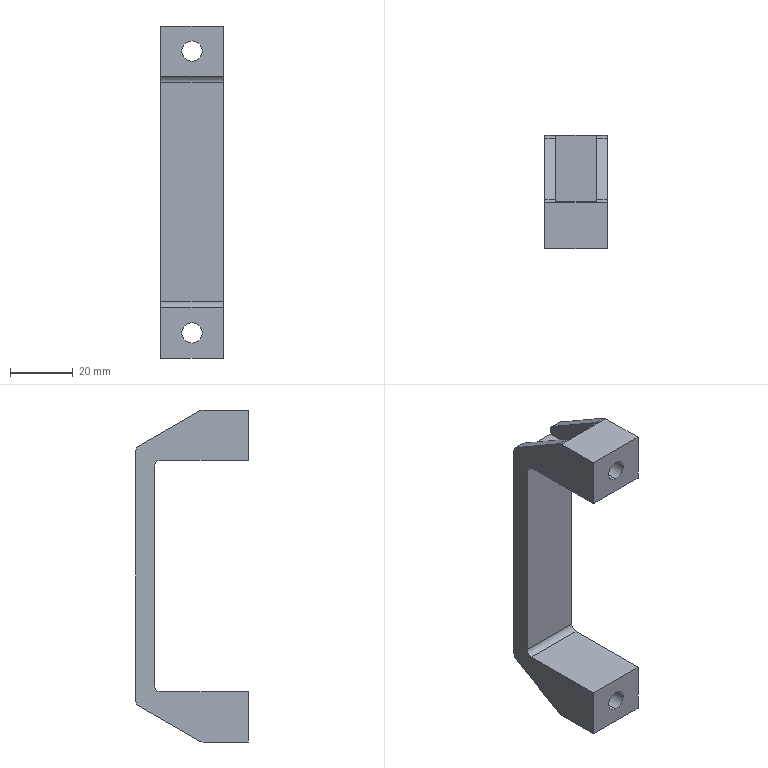Part | SolidWorks | features BaseBody 1 | 1 solid | 40 faces | box 20 x 36 x 106 mm | volume 20303 mm3 | plane 24 | cylinder 16 | commonest cylinder face diameters 4 x8 6.5 x4 11 x4
STEP:
#1=CARTESIAN_POINT('',(10.,15.,50.5));
#2=VERTEX_POINT('',#1);
#3=CARTESIAN_POINT('',(10.,15.,39.5));
#4=VERTEX_POINT('',#3);
#5=CARTESIAN_POINT('',(10.,15.,45.));
#6=DIRECTION('',(0.,-1.,0.));
#7=DIRECTION('',(0.,0.,-1.));
#8=AXIS2_PLACEMENT_3D('',#5,#6,#7);
#9=CIRCLE('',#8,5.5);
#10=EDGE_CURVE('',#2,#4,#9,.T.);
#11=ORIENTED_EDGE('',*,*,#10,.F.);
#12=CARTESIAN_POINT('',(10.,9.5,50.5));
#13=VERTEX_POINT('',#12);
#14=CARTESIAN_POINT('',(10.,15.,50.5));
#15=DIRECTION('',(0.,-1.,0.));
#16=VECTOR('',#15,1000.);
#17=LINE('',#14,#16);
#18=EDGE_CURVE('',#2,#13,#17,.T.);
#19=ORIENTED_EDGE('',*,*,#18,.T.);
#20=CARTESIAN_POINT('',(10.,9.5,39.5));
#21=VERTEX_POINT('',#20);
#22=CARTESIAN_POINT('',(10.,9.5,45.));
#23=DIRECTION('',(0.,1.,0.));
#24=DIRECTION('',(0.,0.,-1.));
#25=AXIS2_PLACEMENT_3D('',#22,#23,#24);
#26=CIRCLE('',#25,5.5);
#27=EDGE_CURVE('',#21,#13,#26,.T.);
#28=ORIENTED_EDGE('',*,*,#27,.F.);
#29=CARTESIAN_POINT('',(10.,15.,39.5));
#30=DIRECTION('',(0.,-1.,0.));
#31=VECTOR('',#30,1000.);
#32=LINE('',#29,#31);
#33=EDGE_CURVE('',#4,#21,#32,.T.);
#34=ORIENTED_EDGE('',*,*,#33,.F.);
#35=EDGE_LOOP('',(#11,#19,#28,#34));
#36=FACE_OUTER_BOUND('',#35,.T.);
#37=CARTESIAN_POINT('',(10.,15.,45.));
#38=DIRECTION('',(0.,-1.,0.));
#39=DIRECTION('',(0.,0.,-1.));
#40=AXIS2_PLACEMENT_3D('',#37,#38,#39);
#41=CYLINDRICAL_SURFACE('',#40,5.5);
#42=ADVANCED_FACE('',(#36),#41,.F.);
#43=CARTESIAN_POINT('',(10.,0.,-41.75));
#44=VERTEX_POINT('',#43);
#45=CARTESIAN_POINT('',(10.,0.,-48.25));
#46=VERTEX_POINT('',#45);
#47=CARTESIAN_POINT('',(10.,0.,-45.));
#48=DIRECTION('',(0.,-1.,0.));
#49=DIRECTION('',(0.,0.,1.));
#50=AXIS2_PLACEMENT_3D('',#47,#48,#49);
#51=CIRCLE('',#50,3.25);
#52=EDGE_CURVE('',#44,#46,#51,.T.);
#53=ORIENTED_EDGE('',*,*,#52,.T.);
#54=CARTESIAN_POINT('',(10.,9.5,-48.25));
#55=VERTEX_POINT('',#54);
#56=CARTESIAN_POINT('',(10.,0.,-48.25));
#57=DIRECTION('',(0.,1.,0.));
#58=VECTOR('',#57,1000.);
#59=LINE('',#56,#58);
#60=EDGE_CURVE('',#46,#55,#59,.T.);
#61=ORIENTED_EDGE('',*,*,#60,.T.);
#62=CARTESIAN_POINT('',(10.,9.5,-41.75));
#63=VERTEX_POINT('',#62);
#64=CARTESIAN_POINT('',(10.,9.5,-45.));
#65=DIRECTION('',(0.,-1.,0.));
#66=DIRECTION('',(0.,0.,1.));
#67=AXIS2_PLACEMENT_3D('',#64,#65,#66);
#68=CIRCLE('',#67,3.25);
#69=EDGE_CURVE('',#63,#55,#68,.T.);
#70=ORIENTED_EDGE('',*,*,#69,.F.);
#71=CARTESIAN_POINT('',(10.,0.,-41.75));
#72=DIRECTION('',(0.,1.,0.));
#73=VECTOR('',#72,1000.);
#74=LINE('',#71,#73);
#75=EDGE_CURVE('',#44,#63,#74,.T.);
#76=ORIENTED_EDGE('',*,*,#75,.F.);
#77=EDGE_LOOP('',(#53,#61,#70,#76));
#78=FACE_OUTER_BOUND('',#77,.T.);
#79=CARTESIAN_POINT('',(10.,0.,-45.));
#80=DIRECTION('',(0.,1.,0.));
#81=DIRECTION('',(0.,0.,1.));
#82=AXIS2_PLACEMENT_3D('',#79,#80,#81);
#83=CYLINDRICAL_SURFACE('',#82,3.25);
#84=ADVANCED_FACE('',(#78),#83,.F.);
#85=CARTESIAN_POINT('',(10.,9.5,48.25));
#86=VERTEX_POINT('',#85);
#87=CARTESIAN_POINT('',(10.,9.5,41.75));
#88=VERTEX_POINT('',#87);
#89=CARTESIAN_POINT('',(10.,9.5,45.));
#90=DIRECTION('',(0.,-1.,0.));
#91=DIRECTION('',(0.,0.,-1.));
#92=AXIS2_PLACEMENT_3D('',#89,#90,#91);
#93=CIRCLE('',#92,3.25);
#94=EDGE_CURVE('',#86,#88,#93,.T.);
#95=ORIENTED_EDGE('',*,*,#94,.F.);
#96=CARTESIAN_POINT('',(10.,0.,48.25));
#97=VERTEX_POINT('',#96);
#98=CARTESIAN_POINT('',(10.,15.,48.25));
#99=DIRECTION('',(0.,-1.,0.));
#100=VECTOR('',#99,1000.);
#101=LINE('',#98,#100);
#102=EDGE_CURVE('',#86,#97,#101,.T.);
#103=ORIENTED_EDGE('',*,*,#102,.T.);
#104=CARTESIAN_POINT('',(10.,0.,41.75));
#105=VERTEX_POINT('',#104);
#106=CARTESIAN_POINT('',(10.,0.,45.));
#107=DIRECTION('',(0.,-1.,0.));
#108=DIRECTION('',(0.,0.,-1.));
#109=AXIS2_PLACEMENT_3D('',#106,#107,#108);
#110=CIRCLE('',#109,3.25);
#111=EDGE_CURVE('',#97,#105,#110,.T.);
#112=ORIENTED_EDGE('',*,*,#111,.T.);
#113=CARTESIAN_POINT('',(10.,15.,41.75));
#114=DIRECTION('',(0.,-1.,0.));
#115=VECTOR('',#114,1000.);
#116=LINE('',#113,#115);
#117=EDGE_CURVE('',#88,#105,#116,.T.);
#118=ORIENTED_EDGE('',*,*,#117,.F.);
#119=EDGE_LOOP('',(#95,#103,#112,#118));
#120=FACE_OUTER_BOUND('',#119,.T.);
#121=CARTESIAN_POINT('',(10.,15.,45.));
#122=DIRECTION('',(0.,-1.,0.));
#123=DIRECTION('',(0.,0.,-1.));
#124=AXIS2_PLACEMENT_3D('',#121,#122,#123);
#125=CYLINDRICAL_SURFACE('',#124,3.25);
#126=ADVANCED_FACE('',(#120),#125,.F.);
#127=CARTESIAN_POINT('',(10.,9.5,-50.5));
#128=VERTEX_POINT('',#127);
#129=CARTESIAN_POINT('',(10.,9.5,-39.5));
#130=VERTEX_POINT('',#129);
#131=CARTESIAN_POINT('',(10.,9.5,-45.));
#132=DIRECTION('',(0.,1.,0.));
#133=DIRECTION('',(0.,0.,1.));
#134=AXIS2_PLACEMENT_3D('',#131,#132,#133);
#135=CIRCLE('',#134,5.5);
#136=EDGE_CURVE('',#128,#130,#135,.T.);
#137=ORIENTED_EDGE('',*,*,#136,.F.);
#138=CARTESIAN_POINT('',(10.,15.,-50.5));
#139=VERTEX_POINT('',#138);
#140=CARTESIAN_POINT('',(10.,0.,-50.5));
#141=DIRECTION('',(0.,1.,0.));
#142=VECTOR('',#141,1000.);
#143=LINE('',#140,#142);
#144=EDGE_CURVE('',#128,#139,#143,.T.);
#145=ORIENTED_EDGE('',*,*,#144,.T.);
#146=CARTESIAN_POINT('',(10.,15.,-39.5));
#147=VERTEX_POINT('',#146);
#148=CARTESIAN_POINT('',(10.,15.,-45.));
#149=DIRECTION('',(0.,-1.,0.));
#150=DIRECTION('',(0.,0.,1.));
#151=AXIS2_PLACEMENT_3D('',#148,#149,#150);
#152=CIRCLE('',#151,5.5);
#153=EDGE_CURVE('',#147,#139,#152,.T.);
#154=ORIENTED_EDGE('',*,*,#153,.F.);
#155=CARTESIAN_POINT('',(10.,0.,-39.5));
#156=DIRECTION('',(0.,1.,0.));
#157=VECTOR('',#156,1000.);
#158=LINE('',#155,#157);
#159=EDGE_CURVE('',#130,#147,#158,.T.);
#160=ORIENTED_EDGE('',*,*,#159,.F.);
#161=EDGE_LOOP('',(#137,#145,#154,#160));
#162=FACE_OUTER_BOUND('',#161,.T.);
#163=CARTESIAN_POINT('',(10.,0.,-45.));
#164=DIRECTION('',(0.,1.,0.));
#165=DIRECTION('',(0.,0.,1.));
#166=AXIS2_PLACEMENT_3D('',#163,#164,#165);
#167=CYLINDRICAL_SURFACE('',#166,5.5);
#168=ADVANCED_FACE('',(#162),#167,.F.);
#169=CARTESIAN_POINT('',(16.5,36.,38.));
#170=VERTEX_POINT('',#169);
#171=CARTESIAN_POINT('',(3.5,36.,38.));
#172=VERTEX_POINT('',#171);
#173=CARTESIAN_POINT('',(20.,36.,38.));
#174=DIRECTION('',(-1.,0.,0.));
#175=VECTOR('',#174,1000.);
#176=LINE('',#173,#175);
#177=EDGE_CURVE('',#170,#172,#176,.T.);
#178=ORIENTED_EDGE('',*,*,#177,.F.);
#179=CARTESIAN_POINT('',(16.5,36.,39.721));
#180=VERTEX_POINT('',#179);
#181=CARTESIAN_POINT('',(16.5,36.,53.));
#182=DIRECTION('',(0.,0.,-1.));
#183=VECTOR('',#182,1000.);
#184=LINE('',#181,#183);
#185=EDGE_CURVE('',#180,#170,#184,.T.);
#186=ORIENTED_EDGE('',*,*,#185,.F.);
#187=CARTESIAN_POINT('',(20.,36.,39.721));
#188=VERTEX_POINT('',#187);
#189=CARTESIAN_POINT('',(20.,36.,39.721));
#190=DIRECTION('',(-1.,0.,0.));
#191=VECTOR('',#190,1000.);
#192=LINE('',#189,#191);
#193=EDGE_CURVE('',#188,#180,#192,.T.);
#194=ORIENTED_EDGE('',*,*,#193,.F.);
#195=CARTESIAN_POINT('',(20.,36.,-39.721));
#196=VERTEX_POINT('',#195);
#197=CARTESIAN_POINT('',(20.,36.,-39.721));
#198=DIRECTION('',(0.,0.,1.));
#199=VECTOR('',#198,1000.);
#200=LINE('',#197,#199);
#201=EDGE_CURVE('',#196,#188,#200,.T.);
#202=ORIENTED_EDGE('',*,*,#201,.F.);
#203=CARTESIAN_POINT('',(16.5,36.,-39.721));
#204=VERTEX_POINT('',#203);
#205=CARTESIAN_POINT('',(20.,36.,-39.721));
#206=DIRECTION('',(1.,0.,0.));
#207=VECTOR('',#206,1000.);
#208=LINE('',#205,#207);
#209=EDGE_CURVE('',#204,#196,#208,.T.);
#210=ORIENTED_EDGE('',*,*,#209,.F.);
#211=CARTESIAN_POINT('',(16.5,36.,-38.));
#212=VERTEX_POINT('',#211);
#213=CARTESIAN_POINT('',(16.5,36.,-38.));
#214=DIRECTION('',(0.,0.,-1.));
#215=VECTOR('',#214,1000.);
#216=LINE('',#213,#215);
#217=EDGE_CURVE('',#212,#204,#216,.T.);
#218=ORIENTED_EDGE('',*,*,#217,.F.);
#219=CARTESIAN_POINT('',(3.5,36.,-38.));
#220=VERTEX_POINT('',#219);
#221=CARTESIAN_POINT('',(20.,36.,-38.));
#222=DIRECTION('',(1.,0.,0.));
#223=VECTOR('',#222,1000.);
#224=LINE('',#221,#223);
#225=EDGE_CURVE('',#220,#212,#224,.T.);
#226=ORIENTED_EDGE('',*,*,#225,.F.);
#227=CARTESIAN_POINT('',(3.5,36.,-39.721));
#228=VERTEX_POINT('',#227);
#229=CARTESIAN_POINT('',(3.5,36.,-53.));
#230=DIRECTION('',(0.,0.,1.));
#231=VECTOR('',#230,1000.);
#232=LINE('',#229,#231);
#233=EDGE_CURVE('',#228,#220,#232,.T.);
#234=ORIENTED_EDGE('',*,*,#233,.F.);
#235=CARTESIAN_POINT('',(0.,36.,-39.721));
#236=VERTEX_POINT('',#235);
#237=CARTESIAN_POINT('',(20.,36.,-39.721));
#238=DIRECTION('',(1.,0.,0.));
#239=VECTOR('',#238,1000.);
#240=LINE('',#237,#239);
#241=EDGE_CURVE('',#236,#228,#240,.T.);
#242=ORIENTED_EDGE('',*,*,#241,.F.);
#243=CARTESIAN_POINT('',(0.,36.,39.721));
#244=VERTEX_POINT('',#243);
#245=CARTESIAN_POINT('',(0.,36.,-39.721));
#246=DIRECTION('',(0.,0.,-1.));
#247=VECTOR('',#246,1000.);
#248=LINE('',#245,#247);
#249=EDGE_CURVE('',#244,#236,#248,.T.);
#250=ORIENTED_EDGE('',*,*,#249,.F.);
#251=CARTESIAN_POINT('',(3.5,36.,39.721));
#252=VERTEX_POINT('',#251);
#253=CARTESIAN_POINT('',(20.,36.,39.721));
#254=DIRECTION('',(-1.,0.,0.));
#255=VECTOR('',#254,1000.);
#256=LINE('',#253,#255);
#257=EDGE_CURVE('',#252,#244,#256,.T.);
#258=ORIENTED_EDGE('',*,*,#257,.F.);
#259=CARTESIAN_POINT('',(3.5,36.,38.));
#260=DIRECTION('',(0.,0.,1.));
#261=VECTOR('',#260,1000.);
#262=LINE('',#259,#261);
#263=EDGE_CURVE('',#172,#252,#262,.T.);
#264=ORIENTED_EDGE('',*,*,#263,.F.);
#265=EDGE_LOOP('',(#178,#186,#194,#202,#210,#218,#226,#234,#242,#250,#258,#264));
#266=FACE_OUTER_BOUND('',#265,.T.);
#267=CARTESIAN_POINT('',(20.,36.,-39.721));
#268=DIRECTION('',(0.,-1.,0.));
#269=DIRECTION('',(0.,0.,-1.));
#270=AXIS2_PLACEMENT_3D('',#267,#268,#269);
#271=PLANE('',#270);
#272=ADVANCED_FACE('',(#266),#271,.F.);
#273=ORIENTED_EDGE('',*,*,#177,.T.);
#274=CARTESIAN_POINT('',(3.5,15.,38.));
#275=VERTEX_POINT('',#274);
#276=CARTESIAN_POINT('',(3.5,36.,38.));
#277=DIRECTION('',(0.,-1.,0.));
#278=VECTOR('',#277,1000.);
#279=LINE('',#276,#278);
#280=EDGE_CURVE('',#172,#275,#279,.T.);
#281=ORIENTED_EDGE('',*,*,#280,.T.);
#282=CARTESIAN_POINT('',(16.5,15.,38.));
#283=VERTEX_POINT('',#282);
#284=CARTESIAN_POINT('',(16.5,15.,38.));
#285=DIRECTION('',(1.,0.,0.));
#286=VECTOR('',#285,1000.);
#287=LINE('',#284,#286);
#288=EDGE_CURVE('',#275,#283,#287,.T.);
#289=ORIENTED_EDGE('',*,*,#288,.T.);
#290=CARTESIAN_POINT('',(16.5,36.,38.));
#291=DIRECTION('',(0.,1.,0.));
#292=VECTOR('',#291,1000.);
#293=LINE('',#290,#292);
#294=EDGE_CURVE('',#283,#170,#293,.T.);
#295=ORIENTED_EDGE('',*,*,#294,.T.);
#296=EDGE_LOOP('',(#273,#281,#289,#295));
#297=FACE_OUTER_BOUND('',#296,.T.);
#298=CARTESIAN_POINT('',(16.5,36.,38.));
#299=DIRECTION('',(0.,0.,1.));
#300=DIRECTION('',(1.,0.,0.));
#301=AXIS2_PLACEMENT_3D('',#298,#299,#300);
#302=PLANE('',#301);
#303=ADVANCED_FACE('',(#297),#302,.T.);
#304=CARTESIAN_POINT('',(20.,35.,41.453));
#305=VERTEX_POINT('',#304);
#306=CARTESIAN_POINT('',(20.,34.,39.721));
#307=DIRECTION('',(-1.,0.,0.));
#308=DIRECTION('',(0.,0.,-1.));
#309=AXIS2_PLACEMENT_3D('',#306,#307,#308);
#310=CIRCLE('',#309,2.);
#311=EDGE_CURVE('',#305,#188,#310,.T.);
#312=ORIENTED_EDGE('',*,*,#311,.T.);
#313=ORIENTED_EDGE('',*,*,#193,.T.);
#314=CARTESIAN_POINT('',(16.5,35.,41.453));
#315=VERTEX_POINT('',#314);
#316=CARTESIAN_POINT('',(16.5,34.,39.721));
#317=DIRECTION('',(1.,0.,0.));
#318=DIRECTION('',(0.,0.,-1.));
#319=AXIS2_PLACEMENT_3D('',#316,#317,#318);
#320=CIRCLE('',#319,2.);
#321=EDGE_CURVE('',#180,#315,#320,.T.);
#322=ORIENTED_EDGE('',*,*,#321,.T.);
#323=CARTESIAN_POINT('',(20.,35.,41.453));
#324=DIRECTION('',(1.,0.,0.));
#325=VECTOR('',#324,1000.);
#326=LINE('',#323,#325);
#327=EDGE_CURVE('',#315,#305,#326,.T.);
#328=ORIENTED_EDGE('',*,*,#327,.T.);
#329=EDGE_LOOP('',(#312,#313,#322,#328));
#330=FACE_OUTER_BOUND('',#329,.T.);
#331=CARTESIAN_POINT('',(20.,34.,39.721));
#332=DIRECTION('',(1.,0.,0.));
#333=DIRECTION('',(0.,0.,-1.));
#334=AXIS2_PLACEMENT_3D('',#331,#332,#333);
#335=CYLINDRICAL_SURFACE('',#334,2.);
#336=ADVANCED_FACE('',(#330),#335,.T.);
#337=ORIENTED_EDGE('',*,*,#311,.F.);
#338=CARTESIAN_POINT('',(20.,15.464,52.732));
#339=VERTEX_POINT('',#338);
#340=CARTESIAN_POINT('',(20.,35.,41.453));
#341=DIRECTION('',(0.,-0.866,0.5));
#342=VECTOR('',#341,1000.);
#343=LINE('',#340,#342);
#344=EDGE_CURVE('',#305,#339,#343,.T.);
#345=ORIENTED_EDGE('',*,*,#344,.T.);
#346=CARTESIAN_POINT('',(20.,14.464,53.));
#347=VERTEX_POINT('',#346);
#348=CARTESIAN_POINT('',(20.,14.464,51.));
#349=DIRECTION('',(-1.,0.,0.));
#350=DIRECTION('',(0.,0.,-1.));
#351=AXIS2_PLACEMENT_3D('',#348,#349,#350);
#352=CIRCLE('',#351,2.);
#353=EDGE_CURVE('',#347,#339,#352,.T.);
#354=ORIENTED_EDGE('',*,*,#353,.F.);
#355=CARTESIAN_POINT('',(20.,0.,53.));
#356=VERTEX_POINT('',#355);
#357=CARTESIAN_POINT('',(20.,14.464,53.));
#358=DIRECTION('',(0.,-1.,0.));
#359=VECTOR('',#358,1000.);
#360=LINE('',#357,#359);
#361=EDGE_CURVE('',#347,#356,#360,.T.);
#362=ORIENTED_EDGE('',*,*,#361,.T.);
#363=CARTESIAN_POINT('',(20.,0.,37.));
#364=VERTEX_POINT('',#363);
#365=CARTESIAN_POINT('',(20.,0.,51.));
#366=DIRECTION('',(0.,0.,-1.));
#367=VECTOR('',#366,1000.);
#368=LINE('',#365,#367);
#369=EDGE_CURVE('',#356,#364,#368,.T.);
#370=ORIENTED_EDGE('',*,*,#369,.T.);
#371=CARTESIAN_POINT('',(20.,28.,37.));
#372=VERTEX_POINT('',#371);
#373=CARTESIAN_POINT('',(20.,14.464,37.));
#374=DIRECTION('',(0.,1.,0.));
#375=VECTOR('',#374,1000.);
#376=LINE('',#373,#375);
#377=EDGE_CURVE('',#364,#372,#376,.T.);
#378=ORIENTED_EDGE('',*,*,#377,.T.);
#379=CARTESIAN_POINT('',(20.,30.,35.));
#380=VERTEX_POINT('',#379);
#381=CARTESIAN_POINT('',(20.,28.,35.));
#382=DIRECTION('',(-1.,0.,0.));
#383=DIRECTION('',(0.,0.,-1.));
#384=AXIS2_PLACEMENT_3D('',#381,#382,#383);
#385=CIRCLE('',#384,2.);
#386=EDGE_CURVE('',#372,#380,#385,.T.);
#387=ORIENTED_EDGE('',*,*,#386,.T.);
#388=CARTESIAN_POINT('',(20.,30.,-35.));
#389=VERTEX_POINT('',#388);
#390=CARTESIAN_POINT('',(20.,30.,51.));
#391=DIRECTION('',(0.,0.,-1.));
#392=VECTOR('',#391,1000.);
#393=LINE('',#390,#392);
#394=EDGE_CURVE('',#380,#389,#393,.T.);
#395=ORIENTED_EDGE('',*,*,#394,.T.);
#396=CARTESIAN_POINT('',(20.,28.,-37.));
#397=VERTEX_POINT('',#396);
#398=CARTESIAN_POINT('',(20.,28.,-35.));
#399=DIRECTION('',(-1.,0.,0.));
#400=DIRECTION('',(0.,0.,-1.));
#401=AXIS2_PLACEMENT_3D('',#398,#399,#400);
#402=CIRCLE('',#401,2.);
#403=EDGE_CURVE('',#389,#397,#402,.T.);
#404=ORIENTED_EDGE('',*,*,#403,.T.);
#405=CARTESIAN_POINT('',(20.,0.,-37.));
#406=VERTEX_POINT('',#405);
#407=CARTESIAN_POINT('',(20.,14.464,-37.));
#408=DIRECTION('',(0.,-1.,0.));
#409=VECTOR('',#408,1000.);
#410=LINE('',#407,#409);
#411=EDGE_CURVE('',#397,#406,#410,.T.);
#412=ORIENTED_EDGE('',*,*,#411,.T.);
#413=CARTESIAN_POINT('',(20.,0.,-53.));
#414=VERTEX_POINT('',#413);
#415=CARTESIAN_POINT('',(20.,0.,51.));
#416=DIRECTION('',(0.,0.,-1.));
#417=VECTOR('',#416,1000.);
#418=LINE('',#415,#417);
#419=EDGE_CURVE('',#406,#414,#418,.T.);
#420=ORIENTED_EDGE('',*,*,#419,.T.);
#421=CARTESIAN_POINT('',(20.,14.464,-53.));
#422=VERTEX_POINT('',#421);
#423=CARTESIAN_POINT('',(20.,14.464,-53.));
#424=DIRECTION('',(0.,1.,0.));
#425=VECTOR('',#424,1000.);
#426=LINE('',#423,#425);
#427=EDGE_CURVE('',#414,#422,#426,.T.);
#428=ORIENTED_EDGE('',*,*,#427,.T.);
#429=CARTESIAN_POINT('',(20.,15.464,-52.732));
#430=VERTEX_POINT('',#429);
#431=CARTESIAN_POINT('',(20.,14.464,-51.));
#432=DIRECTION('',(-1.,0.,0.));
#433=DIRECTION('',(0.,0.,-1.));
#434=AXIS2_PLACEMENT_3D('',#431,#432,#433);
#435=CIRCLE('',#434,2.);
#436=EDGE_CURVE('',#430,#422,#435,.T.);
#437=ORIENTED_EDGE('',*,*,#436,.F.);
#438=CARTESIAN_POINT('',(20.,35.,-41.453));
#439=VERTEX_POINT('',#438);
#440=CARTESIAN_POINT('',(20.,15.464,-52.732));
#441=DIRECTION('',(0.,0.866,0.5));
#442=VECTOR('',#441,1000.);
#443=LINE('',#440,#442);
#444=EDGE_CURVE('',#430,#439,#443,.T.);
#445=ORIENTED_EDGE('',*,*,#444,.T.);
#446=CARTESIAN_POINT('',(20.,34.,-39.721));
#447=DIRECTION('',(1.,0.,0.));
#448=DIRECTION('',(0.,0.,-1.));
#449=AXIS2_PLACEMENT_3D('',#446,#447,#448);
#450=CIRCLE('',#449,2.);
#451=EDGE_CURVE('',#439,#196,#450,.T.);
#452=ORIENTED_EDGE('',*,*,#451,.T.);
#453=ORIENTED_EDGE('',*,*,#201,.T.);
#454=EDGE_LOOP('',(#337,#345,#354,#362,#370,#378,#387,#395,#404,#412,#420,#428,#437,#445,#452,#453));
#455=FACE_OUTER_BOUND('',#454,.T.);
#456=CARTESIAN_POINT('',(20.,14.464,51.));
#457=DIRECTION('',(1.,0.,0.));
#458=DIRECTION('',(0.,0.,-1.));
#459=AXIS2_PLACEMENT_3D('',#456,#457,#458);
#460=PLANE('',#459);
#461=ADVANCED_FACE('',(#455),#460,.T.);
#462=ORIENTED_EDGE('',*,*,#451,.F.);
#463=CARTESIAN_POINT('',(16.5,35.,-41.453));
#464=VERTEX_POINT('',#463);
#465=CARTESIAN_POINT('',(20.,35.,-41.453));
#466=DIRECTION('',(-1.,0.,0.));
#467=VECTOR('',#466,1000.);
#468=LINE('',#465,#467);
#469=EDGE_CURVE('',#439,#464,#468,.T.);
#470=ORIENTED_EDGE('',*,*,#469,.T.);
#471=CARTESIAN_POINT('',(16.5,34.,-39.721));
#472=DIRECTION('',(1.,0.,0.));
#473=DIRECTION('',(0.,0.,-1.));
#474=AXIS2_PLACEMENT_3D('',#471,#472,#473);
#475=CIRCLE('',#474,2.);
#476=EDGE_CURVE('',#464,#204,#475,.T.);
#477=ORIENTED_EDGE('',*,*,#476,.T.);
#478=ORIENTED_EDGE('',*,*,#209,.T.);
#479=EDGE_LOOP('',(#462,#470,#477,#478));
#480=FACE_OUTER_BOUND('',#479,.T.);
#481=CARTESIAN_POINT('',(20.,34.,-39.721));
#482=DIRECTION('',(1.,0.,0.));
#483=DIRECTION('',(0.,0.,-1.));
#484=AXIS2_PLACEMENT_3D('',#481,#482,#483);
#485=CYLINDRICAL_SURFACE('',#484,2.);
#486=ADVANCED_FACE('',(#480),#485,.T.);
#487=ORIENTED_EDGE('',*,*,#225,.T.);
#488=CARTESIAN_POINT('',(16.5,15.,-38.));
#489=VERTEX_POINT('',#488);
#490=CARTESIAN_POINT('',(16.5,36.,-38.));
#491=DIRECTION('',(0.,-1.,0.));
#492=VECTOR('',#491,1000.);
#493=LINE('',#490,#492);
#494=EDGE_CURVE('',#212,#489,#493,.T.);
#495=ORIENTED_EDGE('',*,*,#494,.T.);
#496=CARTESIAN_POINT('',(3.5,15.,-38.));
#497=VERTEX_POINT('',#496);
#498=CARTESIAN_POINT('',(3.5,15.,-38.));
#499=DIRECTION('',(-1.,0.,0.));
#500=VECTOR('',#499,1000.);
#501=LINE('',#498,#500);
#502=EDGE_CURVE('',#489,#497,#501,.T.);
#503=ORIENTED_EDGE('',*,*,#502,.T.);
#504=CARTESIAN_POINT('',(3.5,36.,-38.));
#505=DIRECTION('',(0.,1.,0.));
#506=VECTOR('',#505,1000.);
#507=LINE('',#504,#506);
#508=EDGE_CURVE('',#497,#220,#507,.T.);
#509=ORIENTED_EDGE('',*,*,#508,.T.);
#510=EDGE_LOOP('',(#487,#495,#503,#509));
#511=FACE_OUTER_BOUND('',#510,.T.);
#512=CARTESIAN_POINT('',(3.5,36.,-38.));
#513=DIRECTION('',(0.,0.,-1.));
#514=DIRECTION('',(-1.,0.,0.));
#515=AXIS2_PLACEMENT_3D('',#512,#513,#514);
#516=PLANE('',#515);
#517=ADVANCED_FACE('',(#511),#516,.T.);
#518=CARTESIAN_POINT('',(0.,35.,-41.453));
#519=VERTEX_POINT('',#518);
#520=CARTESIAN_POINT('',(0.,34.,-39.721));
#521=DIRECTION('',(1.,0.,0.));
#522=DIRECTION('',(0.,0.,-1.));
#523=AXIS2_PLACEMENT_3D('',#520,#521,#522);
#524=CIRCLE('',#523,2.);
#525=EDGE_CURVE('',#519,#236,#524,.T.);
#526=ORIENTED_EDGE('',*,*,#525,.T.);
#527=ORIENTED_EDGE('',*,*,#241,.T.);
#528=CARTESIAN_POINT('',(3.5,35.,-41.453));
#529=VERTEX_POINT('',#528);
#530=CARTESIAN_POINT('',(3.5,34.,-39.721));
#531=DIRECTION('',(-1.,0.,0.));
#532=DIRECTION('',(0.,0.,-1.));
#533=AXIS2_PLACEMENT_3D('',#530,#531,#532);
#534=CIRCLE('',#533,2.);
#535=EDGE_CURVE('',#228,#529,#534,.T.);
#536=ORIENTED_EDGE('',*,*,#535,.T.);
#537=CARTESIAN_POINT('',(20.,35.,-41.453));
#538=DIRECTION('',(-1.,0.,0.));
#539=VECTOR('',#538,1000.);
#540=LINE('',#537,#539);
#541=EDGE_CURVE('',#529,#519,#540,.T.);
#542=ORIENTED_EDGE('',*,*,#541,.T.);
#543=EDGE_LOOP('',(#526,#527,#536,#542));
#544=FACE_OUTER_BOUND('',#543,.T.);
#545=CARTESIAN_POINT('',(20.,34.,-39.721));
#546=DIRECTION('',(1.,0.,0.));
#547=DIRECTION('',(0.,0.,-1.));
#548=AXIS2_PLACEMENT_3D('',#545,#546,#547);
#549=CYLINDRICAL_SURFACE('',#548,2.);
#550=ADVANCED_FACE('',(#544),#549,.T.);
#551=CARTESIAN_POINT('',(0.,35.,41.453));
#552=VERTEX_POINT('',#551);
#553=CARTESIAN_POINT('',(0.,15.464,52.732));
#554=VERTEX_POINT('',#553);
#555=CARTESIAN_POINT('',(0.,35.,41.453));
#556=DIRECTION('',(0.,-0.866,0.5));
#557=VECTOR('',#556,1000.);
#558=LINE('',#555,#557);
#559=EDGE_CURVE('',#552,#554,#558,.T.);
#560=ORIENTED_EDGE('',*,*,#559,.F.);
#561=CARTESIAN_POINT('',(0.,34.,39.721));
#562=DIRECTION('',(1.,0.,0.));
#563=DIRECTION('',(0.,0.,-1.));
#564=AXIS2_PLACEMENT_3D('',#561,#562,#563);
#565=CIRCLE('',#564,2.);
#566=EDGE_CURVE('',#244,#552,#565,.T.);
#567=ORIENTED_EDGE('',*,*,#566,.F.);
#568=ORIENTED_EDGE('',*,*,#249,.T.);
#569=ORIENTED_EDGE('',*,*,#525,.F.);
#570=CARTESIAN_POINT('',(0.,15.464,-52.732));
#571=VERTEX_POINT('',#570);
#572=CARTESIAN_POINT('',(0.,15.464,-52.732));
#573=DIRECTION('',(0.,0.866,0.5));
#574=VECTOR('',#573,1000.);
#575=LINE('',#572,#574);
#576=EDGE_CURVE('',#571,#519,#575,.T.);
#577=ORIENTED_EDGE('',*,*,#576,.F.);
#578=CARTESIAN_POINT('',(0.,14.464,-53.));
#579=VERTEX_POINT('',#578);
#580=CARTESIAN_POINT('',(0.,14.464,-51.));
#581=DIRECTION('',(1.,0.,0.));
#582=DIRECTION('',(0.,0.,-1.));
#583=AXIS2_PLACEMENT_3D('',#580,#581,#582);
#584=CIRCLE('',#583,2.);
#585=EDGE_CURVE('',#579,#571,#584,.T.);
#586=ORIENTED_EDGE('',*,*,#585,.F.);
#587=CARTESIAN_POINT('',(0.,0.,-53.));
#588=VERTEX_POINT('',#587);
#589=CARTESIAN_POINT('',(0.,14.464,-53.));
#590=DIRECTION('',(0.,1.,0.));
#591=VECTOR('',#590,1000.);
#592=LINE('',#589,#591);
#593=EDGE_CURVE('',#588,#579,#592,.T.);
#594=ORIENTED_EDGE('',*,*,#593,.F.);
#595=CARTESIAN_POINT('',(0.,0.,-37.));
#596=VERTEX_POINT('',#595);
#597=CARTESIAN_POINT('',(0.,0.,51.));
#598=DIRECTION('',(0.,0.,-1.));
#599=VECTOR('',#598,1000.);
#600=LINE('',#597,#599);
#601=EDGE_CURVE('',#596,#588,#600,.T.);
#602=ORIENTED_EDGE('',*,*,#601,.F.);
#603=CARTESIAN_POINT('',(0.,28.,-37.));
#604=VERTEX_POINT('',#603);
#605=CARTESIAN_POINT('',(0.,14.464,-37.));
#606=DIRECTION('',(0.,-1.,0.));
#607=VECTOR('',#606,1000.);
#608=LINE('',#605,#607);
#609=EDGE_CURVE('',#604,#596,#608,.T.);
#610=ORIENTED_EDGE('',*,*,#609,.F.);
#611=CARTESIAN_POINT('',(0.,30.,-35.));
#612=VERTEX_POINT('',#611);
#613=CARTESIAN_POINT('',(0.,28.,-35.));
#614=DIRECTION('',(-1.,0.,0.));
#615=DIRECTION('',(0.,0.,-1.));
#616=AXIS2_PLACEMENT_3D('',#613,#614,#615);
#617=CIRCLE('',#616,2.);
#618=EDGE_CURVE('',#612,#604,#617,.T.);
#619=ORIENTED_EDGE('',*,*,#618,.F.);
#620=CARTESIAN_POINT('',(0.,30.,35.));
#621=VERTEX_POINT('',#620);
#622=CARTESIAN_POINT('',(0.,30.,51.));
#623=DIRECTION('',(0.,0.,-1.));
#624=VECTOR('',#623,1000.);
#625=LINE('',#622,#624);
#626=EDGE_CURVE('',#621,#612,#625,.T.);
#627=ORIENTED_EDGE('',*,*,#626,.F.);
#628=CARTESIAN_POINT('',(0.,28.,37.));
#629=VERTEX_POINT('',#628);
#630=CARTESIAN_POINT('',(0.,28.,35.));
#631=DIRECTION('',(-1.,0.,0.));
#632=DIRECTION('',(0.,0.,-1.));
#633=AXIS2_PLACEMENT_3D('',#630,#631,#632);
#634=CIRCLE('',#633,2.);
#635=EDGE_CURVE('',#629,#621,#634,.T.);
#636=ORIENTED_EDGE('',*,*,#635,.F.);
#637=CARTESIAN_POINT('',(0.,0.,37.));
#638=VERTEX_POINT('',#637);
#639=CARTESIAN_POINT('',(0.,14.464,37.));
#640=DIRECTION('',(0.,1.,0.));
#641=VECTOR('',#640,1000.);
#642=LINE('',#639,#641);
#643=EDGE_CURVE('',#638,#629,#642,.T.);
#644=ORIENTED_EDGE('',*,*,#643,.F.);
#645=CARTESIAN_POINT('',(0.,0.,53.));
#646=VERTEX_POINT('',#645);
#647=CARTESIAN_POINT('',(0.,0.,51.));
#648=DIRECTION('',(0.,0.,-1.));
#649=VECTOR('',#648,1000.);
#650=LINE('',#647,#649);
#651=EDGE_CURVE('',#646,#638,#650,.T.);
#652=ORIENTED_EDGE('',*,*,#651,.F.);
#653=CARTESIAN_POINT('',(0.,14.464,53.));
#654=VERTEX_POINT('',#653);
#655=CARTESIAN_POINT('',(0.,14.464,53.));
#656=DIRECTION('',(0.,-1.,0.));
#657=VECTOR('',#656,1000.);
#658=LINE('',#655,#657);
#659=EDGE_CURVE('',#654,#646,#658,.T.);
#660=ORIENTED_EDGE('',*,*,#659,.F.);
#661=CARTESIAN_POINT('',(0.,14.464,51.));
#662=DIRECTION('',(1.,0.,0.));
#663=DIRECTION('',(0.,0.,-1.));
#664=AXIS2_PLACEMENT_3D('',#661,#662,#663);
#665=CIRCLE('',#664,2.);
#666=EDGE_CURVE('',#554,#654,#665,.T.);
#667=ORIENTED_EDGE('',*,*,#666,.F.);
#668=EDGE_LOOP('',(#560,#567,#568,#569,#577,#586,#594,#602,#610,#619,#627,#636,#644,#652,#660,#667));
#669=FACE_OUTER_BOUND('',#668,.T.);
#670=CARTESIAN_POINT('',(0.,14.464,51.));
#671=DIRECTION('',(1.,0.,0.));
#672=DIRECTION('',(0.,0.,-1.));
#673=AXIS2_PLACEMENT_3D('',#670,#671,#672);
#674=PLANE('',#673);
#675=ADVANCED_FACE('',(#669),#674,.F.);
#676=ORIENTED_EDGE('',*,*,#566,.T.);
#677=CARTESIAN_POINT('',(3.5,35.,41.453));
#678=VERTEX_POINT('',#677);
#679=CARTESIAN_POINT('',(20.,35.,41.453));
#680=DIRECTION('',(1.,0.,0.));
#681=VECTOR('',#680,1000.);
#682=LINE('',#679,#681);
#683=EDGE_CURVE('',#552,#678,#682,.T.);
#684=ORIENTED_EDGE('',*,*,#683,.T.);
#685=CARTESIAN_POINT('',(3.5,34.,39.721));
#686=DIRECTION('',(-1.,0.,0.));
#687=DIRECTION('',(0.,0.,-1.));
#688=AXIS2_PLACEMENT_3D('',#685,#686,#687);
#689=CIRCLE('',#688,2.);
#690=EDGE_CURVE('',#678,#252,#689,.T.);
#691=ORIENTED_EDGE('',*,*,#690,.T.);
#692=ORIENTED_EDGE('',*,*,#257,.T.);
#693=EDGE_LOOP('',(#676,#684,#691,#692));
#694=FACE_OUTER_BOUND('',#693,.T.);
#695=CARTESIAN_POINT('',(20.,34.,39.721));
#696=DIRECTION('',(1.,0.,0.));
#697=DIRECTION('',(0.,0.,-1.));
#698=AXIS2_PLACEMENT_3D('',#695,#696,#697);
#699=CYLINDRICAL_SURFACE('',#698,2.);
#700=ADVANCED_FACE('',(#694),#699,.T.);
#701=ORIENTED_EDGE('',*,*,#690,.F.);
#702=CARTESIAN_POINT('',(3.5,15.464,52.732));
#703=VERTEX_POINT('',#702);
#704=CARTESIAN_POINT('',(3.5,35.,41.453));
#705=DIRECTION('',(0.,-0.866,0.5));
#706=VECTOR('',#705,1000.);
#707=LINE('',#704,#706);
#708=EDGE_CURVE('',#678,#703,#707,.T.);
#709=ORIENTED_EDGE('',*,*,#708,.T.);
#710=CARTESIAN_POINT('',(3.5,15.,52.927));
#711=VERTEX_POINT('',#710);
#712=CARTESIAN_POINT('',(3.5,14.464,51.));
#713=DIRECTION('',(-1.,0.,0.));
#714=DIRECTION('',(0.,0.,-1.));
#715=AXIS2_PLACEMENT_3D('',#712,#713,#714);
#716=CIRCLE('',#715,2.);
#717=EDGE_CURVE('',#711,#703,#716,.T.);
#718=ORIENTED_EDGE('',*,*,#717,.F.);
#719=CARTESIAN_POINT('',(3.5,15.,38.));
#720=DIRECTION('',(0.,0.,-1.));
#721=VECTOR('',#720,1000.);
#722=LINE('',#719,#721);
#723=EDGE_CURVE('',#711,#275,#722,.T.);
#724=ORIENTED_EDGE('',*,*,#723,.T.);
#725=ORIENTED_EDGE('',*,*,#280,.F.);
#726=ORIENTED_EDGE('',*,*,#263,.T.);
#727=EDGE_LOOP('',(#701,#709,#718,#724,#725,#726));
#728=FACE_OUTER_BOUND('',#727,.T.);
#729=CARTESIAN_POINT('',(3.5,36.,38.));
#730=DIRECTION('',(1.,0.,0.));
#731=DIRECTION('',(0.,0.,-1.));
#732=AXIS2_PLACEMENT_3D('',#729,#730,#731);
#733=PLANE('',#732);
#734=ADVANCED_FACE('',(#728),#733,.T.);
#735=ORIENTED_EDGE('',*,*,#294,.F.);
#736=CARTESIAN_POINT('',(16.5,15.,52.927));
#737=VERTEX_POINT('',#736);
#738=CARTESIAN_POINT('',(16.5,15.,53.));
#739=DIRECTION('',(0.,0.,1.));
#740=VECTOR('',#739,1000.);
#741=LINE('',#738,#740);
#742=EDGE_CURVE('',#283,#737,#741,.T.);
#743=ORIENTED_EDGE('',*,*,#742,.T.);
#744=CARTESIAN_POINT('',(16.5,15.464,52.732));
#745=VERTEX_POINT('',#744);
#746=CARTESIAN_POINT('',(16.5,14.464,51.));
#747=DIRECTION('',(1.,0.,0.));
#748=DIRECTION('',(0.,0.,-1.));
#749=AXIS2_PLACEMENT_3D('',#746,#747,#748);
#750=CIRCLE('',#749,2.);
#751=EDGE_CURVE('',#745,#737,#750,.T.);
#752=ORIENTED_EDGE('',*,*,#751,.F.);
#753=CARTESIAN_POINT('',(16.5,15.464,52.732));
#754=DIRECTION('',(0.,0.866,-0.5));
#755=VECTOR('',#754,1000.);
#756=LINE('',#753,#755);
#757=EDGE_CURVE('',#745,#315,#756,.T.);
#758=ORIENTED_EDGE('',*,*,#757,.T.);
#759=ORIENTED_EDGE('',*,*,#321,.F.);
#760=ORIENTED_EDGE('',*,*,#185,.T.);
#761=EDGE_LOOP('',(#735,#743,#752,#758,#759,#760));
#762=FACE_OUTER_BOUND('',#761,.T.);
#763=CARTESIAN_POINT('',(16.5,36.,53.));
#764=DIRECTION('',(-1.,0.,0.));
#765=DIRECTION('',(0.,0.,1.));
#766=AXIS2_PLACEMENT_3D('',#763,#764,#765);
#767=PLANE('',#766);
#768=ADVANCED_FACE('',(#762),#767,.T.);
#769=ORIENTED_EDGE('',*,*,#288,.F.);
#770=ORIENTED_EDGE('',*,*,#723,.F.);
#771=CARTESIAN_POINT('',(0.,15.,52.927));
#772=DIRECTION('',(1.,0.,0.));
#773=VECTOR('',#772,1000.);
#774=LINE('',#771,#773);
#775=EDGE_CURVE('',#711,#737,#774,.T.);
#776=ORIENTED_EDGE('',*,*,#775,.T.);
#777=ORIENTED_EDGE('',*,*,#742,.F.);
#778=EDGE_LOOP('',(#769,#770,#776,#777));
#779=FACE_OUTER_BOUND('',#778,.T.);
#780=CARTESIAN_POINT('',(10.,15.,45.));
#781=DIRECTION('',(0.,-1.,0.));
#782=DIRECTION('',(0.,0.,-1.));
#783=AXIS2_PLACEMENT_3D('',#780,#781,#782);
#784=CIRCLE('',#783,5.5);
#785=EDGE_CURVE('',#4,#2,#784,.T.);
#786=ORIENTED_EDGE('',*,*,#785,.T.);
#787=ORIENTED_EDGE('',*,*,#10,.T.);
#788=EDGE_LOOP('',(#786,#787));
#789=FACE_BOUND('',#788,.T.);
#790=CARTESIAN_POINT('',(0.,15.,0.));
#791=DIRECTION('',(0.,1.,0.));
#792=DIRECTION('',(0.,0.,1.));
#793=AXIS2_PLACEMENT_3D('',#790,#791,#792);
#794=PLANE('',#793);
#795=ADVANCED_FACE('',(#779,#789),#794,.T.);
#796=CARTESIAN_POINT('',(20.,15.464,52.732));
#797=DIRECTION('',(-1.,0.,0.));
#798=VECTOR('',#797,1000.);
#799=LINE('',#796,#798);
#800=EDGE_CURVE('',#339,#745,#799,.T.);
#801=ORIENTED_EDGE('',*,*,#800,.F.);
#802=ORIENTED_EDGE('',*,*,#344,.F.);
#803=ORIENTED_EDGE('',*,*,#327,.F.);
#804=ORIENTED_EDGE('',*,*,#757,.F.);
#805=EDGE_LOOP('',(#801,#802,#803,#804));
#806=FACE_OUTER_BOUND('',#805,.T.);
#807=CARTESIAN_POINT('',(20.,35.,41.453));
#808=DIRECTION('',(0.,-0.5,-0.866));
#809=DIRECTION('',(0.,0.866,-0.5));
#810=AXIS2_PLACEMENT_3D('',#807,#808,#809);
#811=PLANE('',#810);
#812=ADVANCED_FACE('',(#806),#811,.F.);
#813=ORIENTED_EDGE('',*,*,#469,.F.);
#814=ORIENTED_EDGE('',*,*,#444,.F.);
#815=CARTESIAN_POINT('',(16.5,15.464,-52.732));
#816=VERTEX_POINT('',#815);
#817=CARTESIAN_POINT('',(20.,15.464,-52.732));
#818=DIRECTION('',(1.,0.,0.));
#819=VECTOR('',#818,1000.);
#820=LINE('',#817,#819);
#821=EDGE_CURVE('',#816,#430,#820,.T.);
#822=ORIENTED_EDGE('',*,*,#821,.F.);
#823=CARTESIAN_POINT('',(16.5,15.464,-52.732));
#824=DIRECTION('',(0.,-0.866,-0.5));
#825=VECTOR('',#824,1000.);
#826=LINE('',#823,#825);
#827=EDGE_CURVE('',#464,#816,#826,.T.);
#828=ORIENTED_EDGE('',*,*,#827,.F.);
#829=EDGE_LOOP('',(#813,#814,#822,#828));
#830=FACE_OUTER_BOUND('',#829,.T.);
#831=CARTESIAN_POINT('',(20.,15.464,-52.732));
#832=DIRECTION('',(0.,-0.5,0.866));
#833=DIRECTION('',(0.,-0.866,-0.5));
#834=AXIS2_PLACEMENT_3D('',#831,#832,#833);
#835=PLANE('',#834);
#836=ADVANCED_FACE('',(#830),#835,.F.);
#837=CARTESIAN_POINT('',(20.,14.464,-53.));
#838=DIRECTION('',(-1.,0.,0.));
#839=VECTOR('',#838,1000.);
#840=LINE('',#837,#839);
#841=EDGE_CURVE('',#422,#579,#840,.T.);
#842=ORIENTED_EDGE('',*,*,#841,.F.);
#843=ORIENTED_EDGE('',*,*,#427,.F.);
#844=CARTESIAN_POINT('',(20.,0.,-53.));
#845=DIRECTION('',(1.,0.,0.));
#846=VECTOR('',#845,1000.);
#847=LINE('',#844,#846);
#848=EDGE_CURVE('',#588,#414,#847,.T.);
#849=ORIENTED_EDGE('',*,*,#848,.F.);
#850=ORIENTED_EDGE('',*,*,#593,.T.);
#851=EDGE_LOOP('',(#842,#843,#849,#850));
#852=FACE_OUTER_BOUND('',#851,.T.);
#853=CARTESIAN_POINT('',(20.,0.,-53.));
#854=DIRECTION('',(0.,0.,1.));
#855=DIRECTION('',(1.,0.,0.));
#856=AXIS2_PLACEMENT_3D('',#853,#854,#855);
#857=PLANE('',#856);
#858=ADVANCED_FACE('',(#852),#857,.F.);
#859=ORIENTED_EDGE('',*,*,#848,.T.);
#860=ORIENTED_EDGE('',*,*,#419,.F.);
#861=CARTESIAN_POINT('',(20.,0.,-37.));
#862=DIRECTION('',(1.,0.,0.));
#863=VECTOR('',#862,1000.);
#864=LINE('',#861,#863);
#865=EDGE_CURVE('',#596,#406,#864,.T.);
#866=ORIENTED_EDGE('',*,*,#865,.F.);
#867=ORIENTED_EDGE('',*,*,#601,.T.);
#868=EDGE_LOOP('',(#859,#860,#866,#867));
#869=FACE_OUTER_BOUND('',#868,.T.);
#870=ORIENTED_EDGE('',*,*,#52,.F.);
#871=CARTESIAN_POINT('',(10.,0.,-45.));
#872=DIRECTION('',(0.,-1.,0.));
#873=DIRECTION('',(0.,0.,1.));
#874=AXIS2_PLACEMENT_3D('',#871,#872,#873);
#875=CIRCLE('',#874,3.25);
#876=EDGE_CURVE('',#46,#44,#875,.T.);
#877=ORIENTED_EDGE('',*,*,#876,.F.);
#878=EDGE_LOOP('',(#870,#877));
#879=FACE_BOUND('',#878,.T.);
#880=CARTESIAN_POINT('',(20.,0.,-37.));
#881=DIRECTION('',(0.,1.,0.));
#882=DIRECTION('',(0.,0.,1.));
#883=AXIS2_PLACEMENT_3D('',#880,#881,#882);
#884=PLANE('',#883);
#885=ADVANCED_FACE('',(#869,#879),#884,.F.);
#886=ORIENTED_EDGE('',*,*,#865,.T.);
#887=ORIENTED_EDGE('',*,*,#411,.F.);
#888=CARTESIAN_POINT('',(20.,28.,-37.));
#889=DIRECTION('',(1.,0.,0.));
#890=VECTOR('',#889,1000.);
#891=LINE('',#888,#890);
#892=EDGE_CURVE('',#604,#397,#891,.T.);
#893=ORIENTED_EDGE('',*,*,#892,.F.);
#894=ORIENTED_EDGE('',*,*,#609,.T.);
#895=EDGE_LOOP('',(#886,#887,#893,#894));
#896=FACE_OUTER_BOUND('',#895,.T.);
#897=CARTESIAN_POINT('',(20.,28.,-37.));
#898=DIRECTION('',(0.,0.,-1.));
#899=DIRECTION('',(-1.,0.,0.));
#900=AXIS2_PLACEMENT_3D('',#897,#898,#899);
#901=PLANE('',#900);
#902=ADVANCED_FACE('',(#896),#901,.F.);
#903=ORIENTED_EDGE('',*,*,#892,.T.);
#904=ORIENTED_EDGE('',*,*,#403,.F.);
#905=CARTESIAN_POINT('',(20.,30.,-35.));
#906=DIRECTION('',(1.,0.,0.));
#907=VECTOR('',#906,1000.);
#908=LINE('',#905,#907);
#909=EDGE_CURVE('',#612,#389,#908,.T.);
#910=ORIENTED_EDGE('',*,*,#909,.F.);
#911=ORIENTED_EDGE('',*,*,#618,.T.);
#912=EDGE_LOOP('',(#903,#904,#910,#911));
#913=FACE_OUTER_BOUND('',#912,.T.);
#914=CARTESIAN_POINT('',(20.,28.,-35.));
#915=DIRECTION('',(1.,0.,0.));
#916=DIRECTION('',(0.,0.,-1.));
#917=AXIS2_PLACEMENT_3D('',#914,#915,#916);
#918=CYLINDRICAL_SURFACE('',#917,2.);
#919=ADVANCED_FACE('',(#913),#918,.F.);
#920=ORIENTED_EDGE('',*,*,#909,.T.);
#921=ORIENTED_EDGE('',*,*,#394,.F.);
#922=CARTESIAN_POINT('',(20.,30.,35.));
#923=DIRECTION('',(1.,0.,0.));
#924=VECTOR('',#923,1000.);
#925=LINE('',#922,#924);
#926=EDGE_CURVE('',#621,#380,#925,.T.);
#927=ORIENTED_EDGE('',*,*,#926,.F.);
#928=ORIENTED_EDGE('',*,*,#626,.T.);
#929=EDGE_LOOP('',(#920,#921,#927,#928));
#930=FACE_OUTER_BOUND('',#929,.T.);
#931=CARTESIAN_POINT('',(20.,30.,35.));
#932=DIRECTION('',(0.,1.,0.));
#933=DIRECTION('',(0.,0.,1.));
#934=AXIS2_PLACEMENT_3D('',#931,#932,#933);
#935=PLANE('',#934);
#936=ADVANCED_FACE('',(#930),#935,.F.);
#937=ORIENTED_EDGE('',*,*,#926,.T.);
#938=ORIENTED_EDGE('',*,*,#386,.F.);
#939=CARTESIAN_POINT('',(20.,28.,37.));
#940=DIRECTION('',(1.,0.,0.));
#941=VECTOR('',#940,1000.);
#942=LINE('',#939,#941);
#943=EDGE_CURVE('',#629,#372,#942,.T.);
#944=ORIENTED_EDGE('',*,*,#943,.F.);
#945=ORIENTED_EDGE('',*,*,#635,.T.);
#946=EDGE_LOOP('',(#937,#938,#944,#945));
#947=FACE_OUTER_BOUND('',#946,.T.);
#948=CARTESIAN_POINT('',(20.,28.,35.));
#949=DIRECTION('',(1.,0.,0.));
#950=DIRECTION('',(0.,0.,-1.));
#951=AXIS2_PLACEMENT_3D('',#948,#949,#950);
#952=CYLINDRICAL_SURFACE('',#951,2.);
#953=ADVANCED_FACE('',(#947),#952,.F.);
#954=ORIENTED_EDGE('',*,*,#943,.T.);
#955=ORIENTED_EDGE('',*,*,#377,.F.);
#956=CARTESIAN_POINT('',(20.,0.,37.));
#957=DIRECTION('',(1.,0.,0.));
#958=VECTOR('',#957,1000.);
#959=LINE('',#956,#958);
#960=EDGE_CURVE('',#638,#364,#959,.T.);
#961=ORIENTED_EDGE('',*,*,#960,.F.);
#962=ORIENTED_EDGE('',*,*,#643,.T.);
#963=EDGE_LOOP('',(#954,#955,#961,#962));
#964=FACE_OUTER_BOUND('',#963,.T.);
#965=CARTESIAN_POINT('',(20.,0.,37.));
#966=DIRECTION('',(0.,0.,1.));
#967=DIRECTION('',(1.,0.,0.));
#968=AXIS2_PLACEMENT_3D('',#965,#966,#967);
#969=PLANE('',#968);
#970=ADVANCED_FACE('',(#964),#969,.F.);
#971=ORIENTED_EDGE('',*,*,#960,.T.);
#972=ORIENTED_EDGE('',*,*,#369,.F.);
#973=CARTESIAN_POINT('',(20.,0.,53.));
#974=DIRECTION('',(1.,0.,0.));
#975=VECTOR('',#974,1000.);
#976=LINE('',#973,#975);
#977=EDGE_CURVE('',#646,#356,#976,.T.);
#978=ORIENTED_EDGE('',*,*,#977,.F.);
#979=ORIENTED_EDGE('',*,*,#651,.T.);
#980=EDGE_LOOP('',(#971,#972,#978,#979));
#981=FACE_OUTER_BOUND('',#980,.T.);
#982=CARTESIAN_POINT('',(10.,0.,45.));
#983=DIRECTION('',(0.,-1.,0.));
#984=DIRECTION('',(0.,0.,-1.));
#985=AXIS2_PLACEMENT_3D('',#982,#983,#984);
#986=CIRCLE('',#985,3.25);
#987=EDGE_CURVE('',#105,#97,#986,.T.);
#988=ORIENTED_EDGE('',*,*,#987,.F.);
#989=ORIENTED_EDGE('',*,*,#111,.F.);
#990=EDGE_LOOP('',(#988,#989));
#991=FACE_BOUND('',#990,.T.);
#992=CARTESIAN_POINT('',(20.,0.,53.));
#993=DIRECTION('',(0.,1.,0.));
#994=DIRECTION('',(0.,0.,1.));
#995=AXIS2_PLACEMENT_3D('',#992,#993,#994);
#996=PLANE('',#995);
#997=ADVANCED_FACE('',(#981,#991),#996,.F.);
#998=ORIENTED_EDGE('',*,*,#977,.T.);
#999=ORIENTED_EDGE('',*,*,#361,.F.);
#1000=CARTESIAN_POINT('',(20.,14.464,53.));
#1001=DIRECTION('',(1.,0.,0.));
#1002=VECTOR('',#1001,1000.);
#1003=LINE('',#1000,#1002);
#1004=EDGE_CURVE('',#654,#347,#1003,.T.);
#1005=ORIENTED_EDGE('',*,*,#1004,.F.);
#1006=ORIENTED_EDGE('',*,*,#659,.T.);
#1007=EDGE_LOOP('',(#998,#999,#1005,#1006));
#1008=FACE_OUTER_BOUND('',#1007,.T.);
#1009=CARTESIAN_POINT('',(20.,14.464,53.));
#1010=DIRECTION('',(0.,0.,-1.));
#1011=DIRECTION('',(-1.,0.,0.));
#1012=AXIS2_PLACEMENT_3D('',#1009,#1010,#1011);
#1013=PLANE('',#1012);
#1014=ADVANCED_FACE('',(#1008),#1013,.F.);
#1015=ORIENTED_EDGE('',*,*,#476,.F.);
#1016=ORIENTED_EDGE('',*,*,#827,.T.);
#1017=CARTESIAN_POINT('',(16.5,15.,-52.927));
#1018=VERTEX_POINT('',#1017);
#1019=CARTESIAN_POINT('',(16.5,14.464,-51.));
#1020=DIRECTION('',(-1.,0.,0.));
#1021=DIRECTION('',(0.,0.,-1.));
#1022=AXIS2_PLACEMENT_3D('',#1019,#1020,#1021);
#1023=CIRCLE('',#1022,2.);
#1024=EDGE_CURVE('',#816,#1018,#1023,.T.);
#1025=ORIENTED_EDGE('',*,*,#1024,.T.);
#1026=CARTESIAN_POINT('',(16.5,15.,-38.));
#1027=DIRECTION('',(0.,0.,1.));
#1028=VECTOR('',#1027,1000.);
#1029=LINE('',#1026,#1028);
#1030=EDGE_CURVE('',#1018,#489,#1029,.T.);
#1031=ORIENTED_EDGE('',*,*,#1030,.T.);
#1032=ORIENTED_EDGE('',*,*,#494,.F.);
#1033=ORIENTED_EDGE('',*,*,#217,.T.);
#1034=EDGE_LOOP('',(#1015,#1016,#1025,#1031,#1032,#1033));
#1035=FACE_OUTER_BOUND('',#1034,.T.);
#1036=CARTESIAN_POINT('',(16.5,36.,-38.));
#1037=DIRECTION('',(-1.,0.,0.));
#1038=DIRECTION('',(0.,0.,1.));
#1039=AXIS2_PLACEMENT_3D('',#1036,#1037,#1038);
#1040=PLANE('',#1039);
#1041=ADVANCED_FACE('',(#1035),#1040,.T.);
#1042=ORIENTED_EDGE('',*,*,#508,.F.);
#1043=CARTESIAN_POINT('',(3.5,15.,-52.927));
#1044=VERTEX_POINT('',#1043);
#1045=CARTESIAN_POINT('',(3.5,15.,-53.));
#1046=DIRECTION('',(0.,0.,-1.));
#1047=VECTOR('',#1046,1000.);
#1048=LINE('',#1045,#1047);
#1049=EDGE_CURVE('',#497,#1044,#1048,.T.);
#1050=ORIENTED_EDGE('',*,*,#1049,.T.);
#1051=CARTESIAN_POINT('',(3.5,15.464,-52.732));
#1052=VERTEX_POINT('',#1051);
#1053=CARTESIAN_POINT('',(3.5,14.464,-51.));
#1054=DIRECTION('',(1.,0.,0.));
#1055=DIRECTION('',(0.,0.,-1.));
#1056=AXIS2_PLACEMENT_3D('',#1053,#1054,#1055);
#1057=CIRCLE('',#1056,2.);
#1058=EDGE_CURVE('',#1044,#1052,#1057,.T.);
#1059=ORIENTED_EDGE('',*,*,#1058,.T.);
#1060=CARTESIAN_POINT('',(3.5,15.464,-52.732));
#1061=DIRECTION('',(0.,0.866,0.5));
#1062=VECTOR('',#1061,1000.);
#1063=LINE('',#1060,#1062);
#1064=EDGE_CURVE('',#1052,#529,#1063,.T.);
#1065=ORIENTED_EDGE('',*,*,#1064,.T.);
#1066=ORIENTED_EDGE('',*,*,#535,.F.);
#1067=ORIENTED_EDGE('',*,*,#233,.T.);
#1068=EDGE_LOOP('',(#1042,#1050,#1059,#1065,#1066,#1067));
#1069=FACE_OUTER_BOUND('',#1068,.T.);
#1070=CARTESIAN_POINT('',(3.5,36.,-53.));
#1071=DIRECTION('',(1.,0.,0.));
#1072=DIRECTION('',(0.,0.,-1.));
#1073=AXIS2_PLACEMENT_3D('',#1070,#1071,#1072);
#1074=PLANE('',#1073);
#1075=ADVANCED_FACE('',(#1069),#1074,.T.);
#1076=ORIENTED_EDGE('',*,*,#502,.F.);
#1077=ORIENTED_EDGE('',*,*,#1030,.F.);
#1078=CARTESIAN_POINT('',(0.,15.,-52.927));
#1079=DIRECTION('',(-1.,0.,0.));
#1080=VECTOR('',#1079,1000.);
#1081=LINE('',#1078,#1080);
#1082=EDGE_CURVE('',#1018,#1044,#1081,.T.);
#1083=ORIENTED_EDGE('',*,*,#1082,.T.);
#1084=ORIENTED_EDGE('',*,*,#1049,.F.);
#1085=EDGE_LOOP('',(#1076,#1077,#1083,#1084));
#1086=FACE_OUTER_BOUND('',#1085,.T.);
#1087=ORIENTED_EDGE('',*,*,#153,.T.);
#1088=CARTESIAN_POINT('',(10.,15.,-45.));
#1089=DIRECTION('',(0.,-1.,0.));
#1090=DIRECTION('',(0.,0.,1.));
#1091=AXIS2_PLACEMENT_3D('',#1088,#1089,#1090);
#1092=CIRCLE('',#1091,5.5);
#1093=EDGE_CURVE('',#139,#147,#1092,.T.);
#1094=ORIENTED_EDGE('',*,*,#1093,.T.);
#1095=EDGE_LOOP('',(#1087,#1094));
#1096=FACE_BOUND('',#1095,.T.);
#1097=CARTESIAN_POINT('',(0.,15.,0.));
#1098=DIRECTION('',(0.,1.,0.));
#1099=DIRECTION('',(0.,0.,1.));
#1100=AXIS2_PLACEMENT_3D('',#1097,#1098,#1099);
#1101=PLANE('',#1100);
#1102=ADVANCED_FACE('',(#1086,#1096),#1101,.T.);
#1103=CARTESIAN_POINT('',(20.,15.464,-52.732));
#1104=DIRECTION('',(1.,0.,0.));
#1105=VECTOR('',#1104,1000.);
#1106=LINE('',#1103,#1105);
#1107=EDGE_CURVE('',#571,#1052,#1106,.T.);
#1108=ORIENTED_EDGE('',*,*,#1107,.F.);
#1109=ORIENTED_EDGE('',*,*,#576,.T.);
#1110=ORIENTED_EDGE('',*,*,#541,.F.);
#1111=ORIENTED_EDGE('',*,*,#1064,.F.);
#1112=EDGE_LOOP('',(#1108,#1109,#1110,#1111));
#1113=FACE_OUTER_BOUND('',#1112,.T.);
#1114=CARTESIAN_POINT('',(20.,15.464,-52.732));
#1115=DIRECTION('',(0.,-0.5,0.866));
#1116=DIRECTION('',(0.,-0.866,-0.5));
#1117=AXIS2_PLACEMENT_3D('',#1114,#1115,#1116);
#1118=PLANE('',#1117);
#1119=ADVANCED_FACE('',(#1113),#1118,.F.);
#1120=ORIENTED_EDGE('',*,*,#683,.F.);
#1121=ORIENTED_EDGE('',*,*,#559,.T.);
#1122=CARTESIAN_POINT('',(20.,15.464,52.732));
#1123=DIRECTION('',(-1.,0.,0.));
#1124=VECTOR('',#1123,1000.);
#1125=LINE('',#1122,#1124);
#1126=EDGE_CURVE('',#703,#554,#1125,.T.);
#1127=ORIENTED_EDGE('',*,*,#1126,.F.);
#1128=ORIENTED_EDGE('',*,*,#708,.F.);
#1129=EDGE_LOOP('',(#1120,#1121,#1127,#1128));
#1130=FACE_OUTER_BOUND('',#1129,.T.);
#1131=CARTESIAN_POINT('',(20.,35.,41.453));
#1132=DIRECTION('',(0.,-0.5,-0.866));
#1133=DIRECTION('',(0.,0.866,-0.5));
#1134=AXIS2_PLACEMENT_3D('',#1131,#1132,#1133);
#1135=PLANE('',#1134);
#1136=ADVANCED_FACE('',(#1130),#1135,.F.);
#1137=ORIENTED_EDGE('',*,*,#751,.T.);
#1138=ORIENTED_EDGE('',*,*,#775,.F.);
#1139=ORIENTED_EDGE('',*,*,#717,.T.);
#1140=ORIENTED_EDGE('',*,*,#1126,.T.);
#1141=ORIENTED_EDGE('',*,*,#666,.T.);
#1142=ORIENTED_EDGE('',*,*,#1004,.T.);
#1143=ORIENTED_EDGE('',*,*,#353,.T.);
#1144=ORIENTED_EDGE('',*,*,#800,.T.);
#1145=EDGE_LOOP('',(#1137,#1138,#1139,#1140,#1141,#1142,#1143,#1144));
#1146=FACE_OUTER_BOUND('',#1145,.T.);
#1147=CARTESIAN_POINT('',(20.,14.464,51.));
#1148=DIRECTION('',(1.,0.,0.));
#1149=DIRECTION('',(0.,0.,-1.));
#1150=AXIS2_PLACEMENT_3D('',#1147,#1148,#1149);
#1151=CYLINDRICAL_SURFACE('',#1150,2.);
#1152=ADVANCED_FACE('',(#1146),#1151,.T.);
#1153=ORIENTED_EDGE('',*,*,#18,.F.);
#1154=ORIENTED_EDGE('',*,*,#785,.F.);
#1155=ORIENTED_EDGE('',*,*,#33,.T.);
#1156=CARTESIAN_POINT('',(10.,9.5,45.));
#1157=DIRECTION('',(0.,1.,0.));
#1158=DIRECTION('',(0.,0.,-1.));
#1159=AXIS2_PLACEMENT_3D('',#1156,#1157,#1158);
#1160=CIRCLE('',#1159,5.5);
#1161=EDGE_CURVE('',#13,#21,#1160,.T.);
#1162=ORIENTED_EDGE('',*,*,#1161,.F.);
#1163=EDGE_LOOP('',(#1153,#1154,#1155,#1162));
#1164=FACE_OUTER_BOUND('',#1163,.T.);
#1165=CARTESIAN_POINT('',(10.,15.,45.));
#1166=DIRECTION('',(0.,-1.,0.));
#1167=DIRECTION('',(0.,0.,-1.));
#1168=AXIS2_PLACEMENT_3D('',#1165,#1166,#1167);
#1169=CYLINDRICAL_SURFACE('',#1168,5.5);
#1170=ADVANCED_FACE('',(#1164),#1169,.F.);
#1171=ORIENTED_EDGE('',*,*,#585,.T.);
#1172=ORIENTED_EDGE('',*,*,#1107,.T.);
#1173=ORIENTED_EDGE('',*,*,#1058,.F.);
#1174=ORIENTED_EDGE('',*,*,#1082,.F.);
#1175=ORIENTED_EDGE('',*,*,#1024,.F.);
#1176=ORIENTED_EDGE('',*,*,#821,.T.);
#1177=ORIENTED_EDGE('',*,*,#436,.T.);
#1178=ORIENTED_EDGE('',*,*,#841,.T.);
#1179=EDGE_LOOP('',(#1171,#1172,#1173,#1174,#1175,#1176,#1177,#1178));
#1180=FACE_OUTER_BOUND('',#1179,.T.);
#1181=CARTESIAN_POINT('',(20.,14.464,-51.));
#1182=DIRECTION('',(1.,0.,0.));
#1183=DIRECTION('',(0.,0.,-1.));
#1184=AXIS2_PLACEMENT_3D('',#1181,#1182,#1183);
#1185=CYLINDRICAL_SURFACE('',#1184,2.);
#1186=ADVANCED_FACE('',(#1180),#1185,.T.);
#1187=ORIENTED_EDGE('',*,*,#60,.F.);
#1188=ORIENTED_EDGE('',*,*,#876,.T.);
#1189=ORIENTED_EDGE('',*,*,#75,.T.);
#1190=CARTESIAN_POINT('',(10.,9.5,-45.));
#1191=DIRECTION('',(0.,-1.,0.));
#1192=DIRECTION('',(0.,0.,1.));
#1193=AXIS2_PLACEMENT_3D('',#1190,#1191,#1192);
#1194=CIRCLE('',#1193,3.25);
#1195=EDGE_CURVE('',#55,#63,#1194,.T.);
#1196=ORIENTED_EDGE('',*,*,#1195,.F.);
#1197=EDGE_LOOP('',(#1187,#1188,#1189,#1196));
#1198=FACE_OUTER_BOUND('',#1197,.T.);
#1199=CARTESIAN_POINT('',(10.,0.,-45.));
#1200=DIRECTION('',(0.,1.,0.));
#1201=DIRECTION('',(0.,0.,1.));
#1202=AXIS2_PLACEMENT_3D('',#1199,#1200,#1201);
#1203=CYLINDRICAL_SURFACE('',#1202,3.25);
#1204=ADVANCED_FACE('',(#1198),#1203,.F.);
#1205=ORIENTED_EDGE('',*,*,#102,.F.);
#1206=CARTESIAN_POINT('',(10.,9.5,45.));
#1207=DIRECTION('',(0.,-1.,0.));
#1208=DIRECTION('',(0.,0.,-1.));
#1209=AXIS2_PLACEMENT_3D('',#1206,#1207,#1208);
#1210=CIRCLE('',#1209,3.25);
#1211=EDGE_CURVE('',#88,#86,#1210,.T.);
#1212=ORIENTED_EDGE('',*,*,#1211,.F.);
#1213=ORIENTED_EDGE('',*,*,#117,.T.);
#1214=ORIENTED_EDGE('',*,*,#987,.T.);
#1215=EDGE_LOOP('',(#1205,#1212,#1213,#1214));
#1216=FACE_OUTER_BOUND('',#1215,.T.);
#1217=CARTESIAN_POINT('',(10.,15.,45.));
#1218=DIRECTION('',(0.,-1.,0.));
#1219=DIRECTION('',(0.,0.,-1.));
#1220=AXIS2_PLACEMENT_3D('',#1217,#1218,#1219);
#1221=CYLINDRICAL_SURFACE('',#1220,3.25);
#1222=ADVANCED_FACE('',(#1216),#1221,.F.);
#1223=ORIENTED_EDGE('',*,*,#144,.F.);
#1224=CARTESIAN_POINT('',(10.,9.5,-45.));
#1225=DIRECTION('',(0.,1.,0.));
#1226=DIRECTION('',(0.,0.,1.));
#1227=AXIS2_PLACEMENT_3D('',#1224,#1225,#1226);
#1228=CIRCLE('',#1227,5.5);
#1229=EDGE_CURVE('',#130,#128,#1228,.T.);
#1230=ORIENTED_EDGE('',*,*,#1229,.F.);
#1231=ORIENTED_EDGE('',*,*,#159,.T.);
#1232=ORIENTED_EDGE('',*,*,#1093,.F.);
#1233=EDGE_LOOP('',(#1223,#1230,#1231,#1232));
#1234=FACE_OUTER_BOUND('',#1233,.T.);
#1235=CARTESIAN_POINT('',(10.,0.,-45.));
#1236=DIRECTION('',(0.,1.,0.));
#1237=DIRECTION('',(0.,0.,1.));
#1238=AXIS2_PLACEMENT_3D('',#1235,#1236,#1237);
#1239=CYLINDRICAL_SURFACE('',#1238,5.5);
#1240=ADVANCED_FACE('',(#1234),#1239,.F.);
#1241=ORIENTED_EDGE('',*,*,#1211,.T.);
#1242=ORIENTED_EDGE('',*,*,#94,.T.);
#1243=EDGE_LOOP('',(#1241,#1242));
#1244=FACE_BOUND('',#1243,.T.);
#1245=ORIENTED_EDGE('',*,*,#27,.T.);
#1246=ORIENTED_EDGE('',*,*,#1161,.T.);
#1247=EDGE_LOOP('',(#1245,#1246));
#1248=FACE_OUTER_BOUND('',#1247,.T.);
#1249=CARTESIAN_POINT('',(10.,9.5,48.25));
#1250=DIRECTION('',(0.,1.,0.));
#1251=DIRECTION('',(0.,0.,1.));
#1252=AXIS2_PLACEMENT_3D('',#1249,#1250,#1251);
#1253=PLANE('',#1252);
#1254=ADVANCED_FACE('',(#1244,#1248),#1253,.T.);
#1255=ORIENTED_EDGE('',*,*,#1229,.T.);
#1256=ORIENTED_EDGE('',*,*,#136,.T.);
#1257=EDGE_LOOP('',(#1255,#1256));
#1258=FACE_OUTER_BOUND('',#1257,.T.);
#1259=ORIENTED_EDGE('',*,*,#69,.T.);
#1260=ORIENTED_EDGE('',*,*,#1195,.T.);
#1261=EDGE_LOOP('',(#1259,#1260));
#1262=FACE_BOUND('',#1261,.T.);
#1263=CARTESIAN_POINT('',(10.,9.5,-50.5));
#1264=DIRECTION('',(0.,1.,0.));
#1265=DIRECTION('',(0.,0.,1.));
#1266=AXIS2_PLACEMENT_3D('',#1263,#1264,#1265);
#1267=PLANE('',#1266);
#1268=ADVANCED_FACE('',(#1258,#1262),#1267,.T.);
#1269=CLOSED_SHELL('',(#42,#84,#126,#168,#272,#303,#336,#461,#486,#517,#550,#675,#700,#734,#768,#795,#812,#836,#858,#885,#902,#919,#936,#953,#970,#997,#1014,#1041,#1075,#1102,#1119,#1136,#1152,#1170,#1186,#1204,#1222,#1240,#1254,#1268));
#1270=MANIFOLD_SOLID_BREP('',#1269);
#1271=CARTESIAN_POINT('',(0.,0.,0.));
#1272=DIRECTION('',(0.,0.,1.));
#1273=DIRECTION('',(1.,0.,0.));
#1274=AXIS2_PLACEMENT_3D('',#1271,#1272,#1273);
#1275=(LENGTH_UNIT()NAMED_UNIT(*)SI_UNIT(.MILLI.,.METRE.));
#1276=UNCERTAINTY_MEASURE_WITH_UNIT(LENGTH_MEASURE(0.00001),#1275,'','');
#1277=(NAMED_UNIT(*)PLANE_ANGLE_UNIT()SI_UNIT($,.RADIAN.));
#1278=(NAMED_UNIT(*)SI_UNIT($,.STERADIAN.)SOLID_ANGLE_UNIT());
#1279=(GEOMETRIC_REPRESENTATION_CONTEXT(3)GLOBAL_UNCERTAINTY_ASSIGNED_CONTEXT((#1276))GLOBAL_UNIT_ASSIGNED_CONTEXT((#1275,#1277,#1278))REPRESENTATION_CONTEXT('',''));
#1280=ADVANCED_BREP_SHAPE_REPRESENTATION('',(#1270,#1274),#1279);